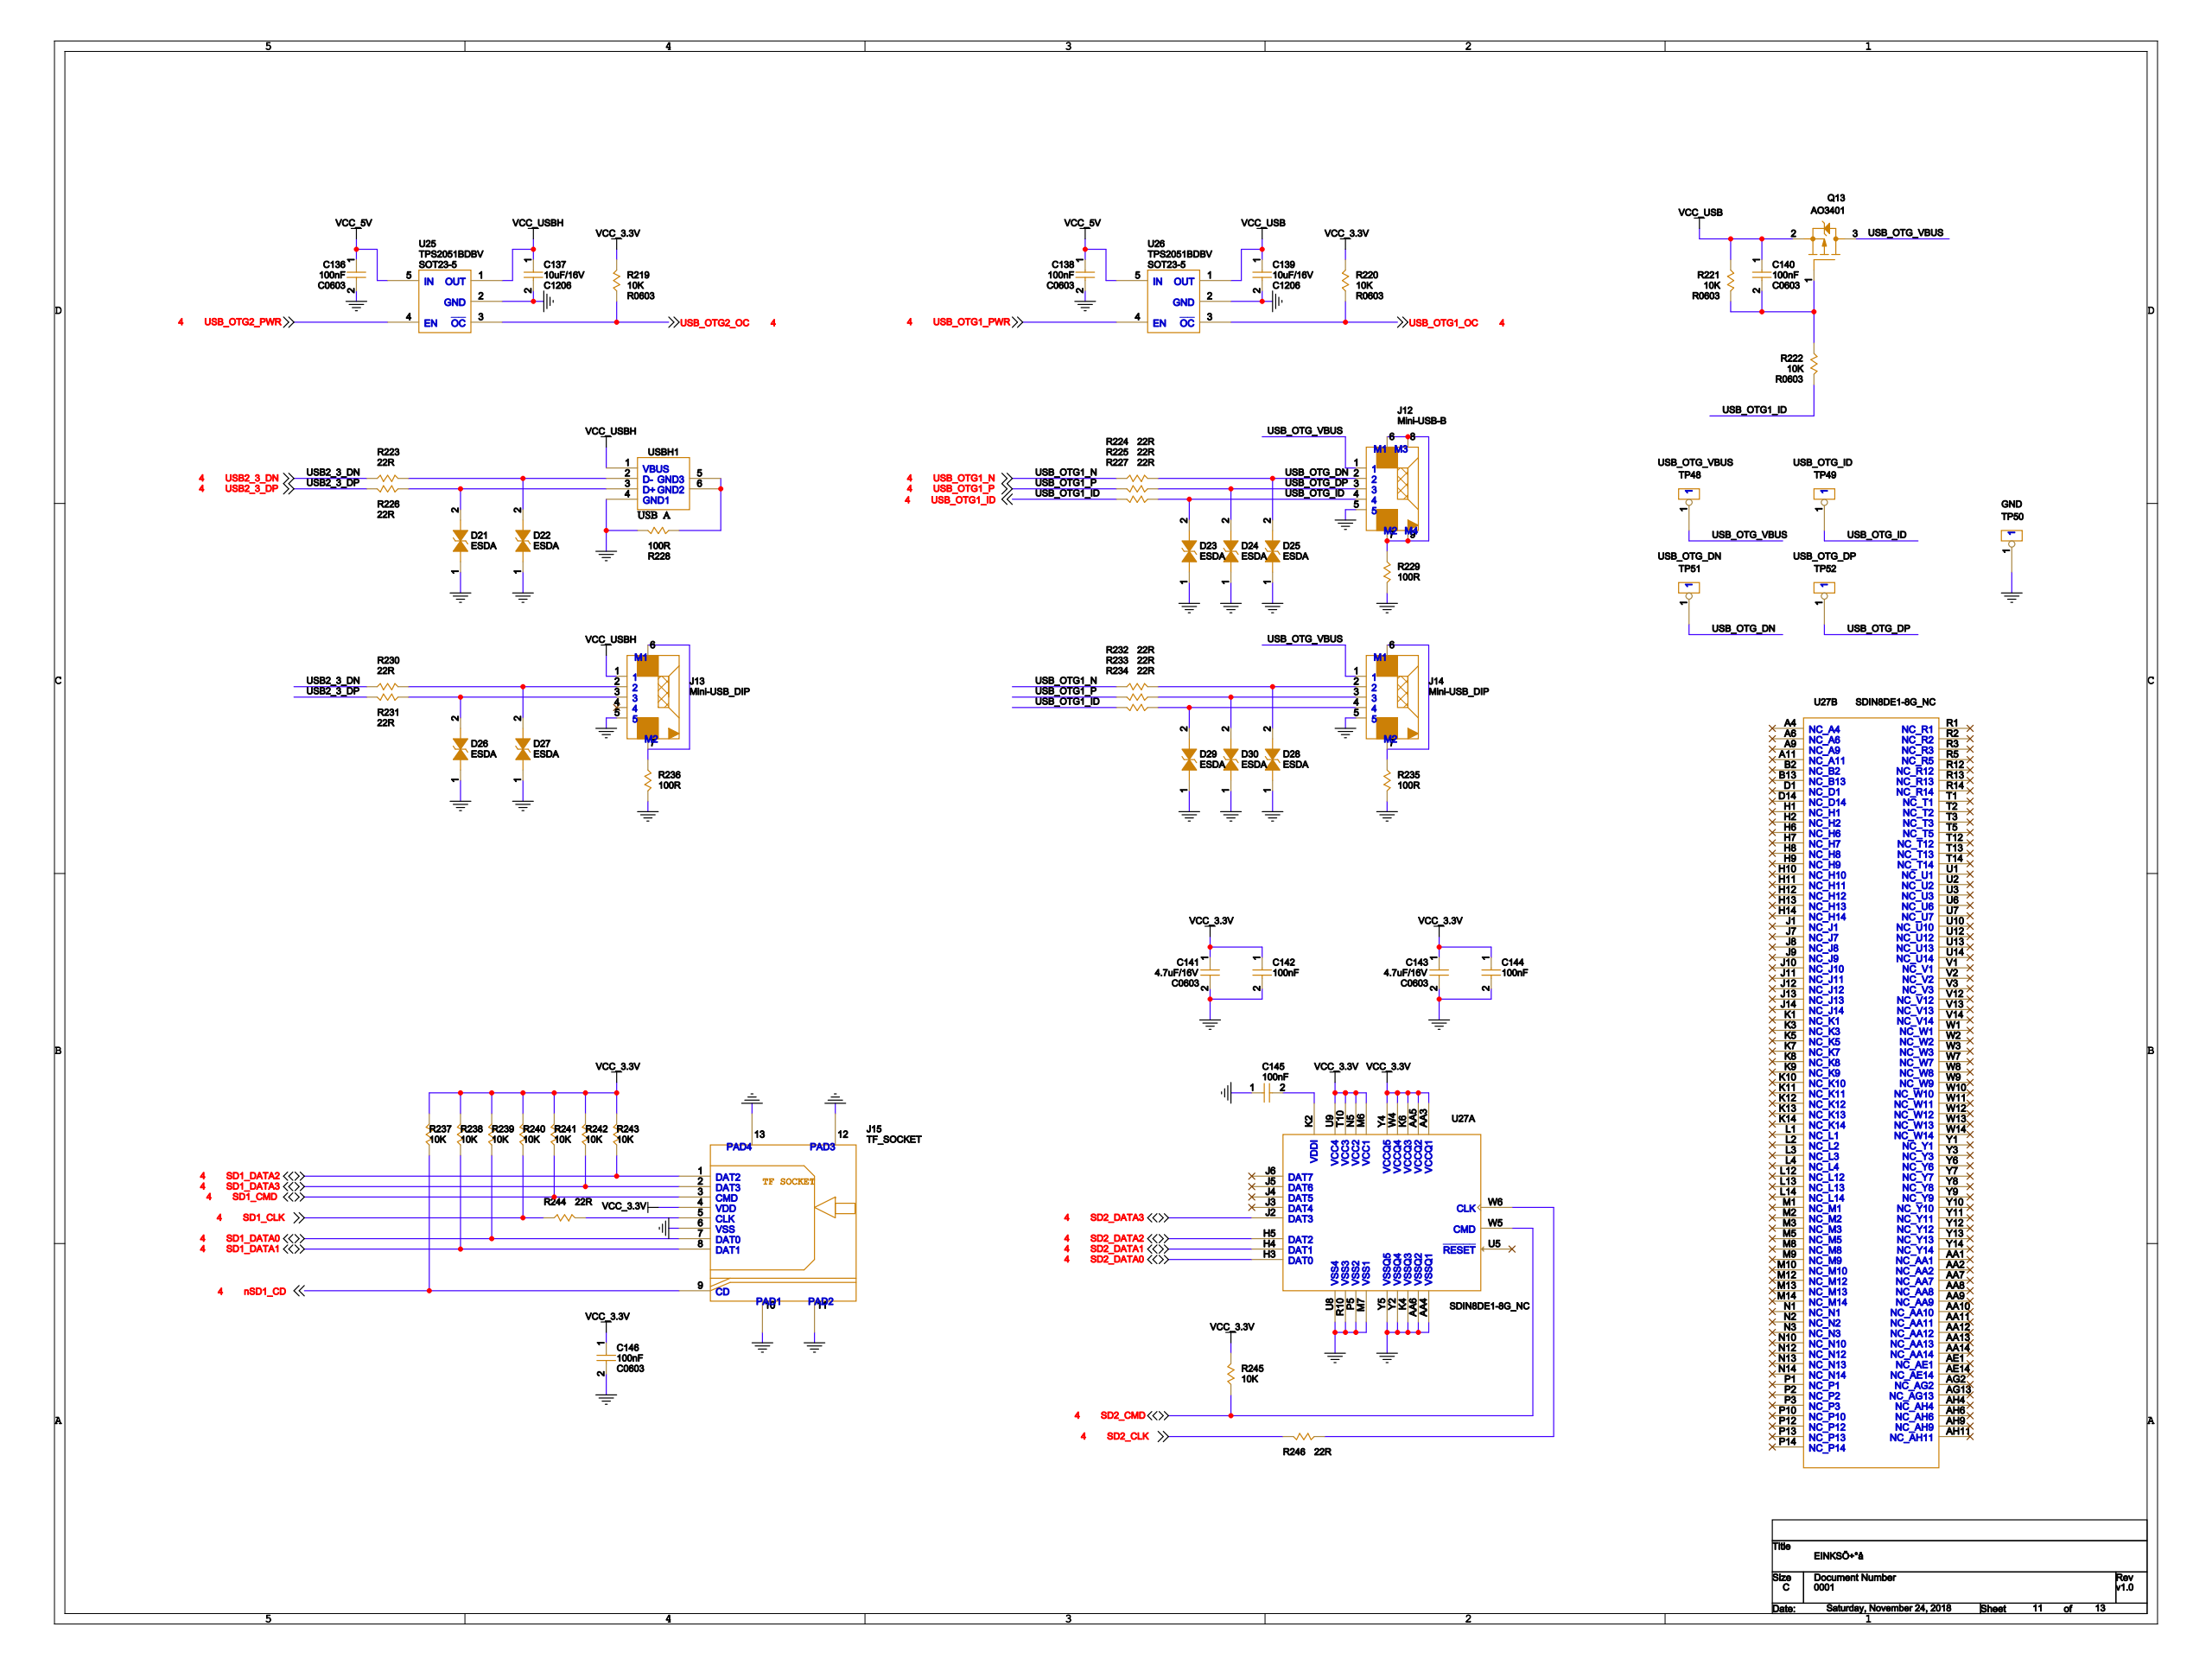Circuit board | Cadence Allegro | 609 parts | 409 nets | one sheet of the schematic
Parts on this sheet (reference | value | footprint):
C136 | 100nF | C0603
C137 | 10uF/16V | C1206
C138 | 100nF | C0603
C139 | 10uF/16V | C1206
C140 | 100nF | C0603
C141 | 4.7uF/16V | C0603
C142 | 100nF | C0603
C143 | 4.7uF/16V | C0603
C144 | 100nF | C0603
C145 | 100nF | C0603
C146 | 100nF | C0603
D21 | ESDA | 0603ESDA
D22 | ESDA | 0603ESDA
D23 | ESDA | 0603ESDA
D24 | ESDA | 0603ESDA
D25 | ESDA | 0603ESDA
D26 | ESDA | 0603ESDA
D27 | ESDA | 0603ESDA
D28 | ESDA | 0603ESDA
D29 | ESDA | 0603ESDA
D30 | ESDA | 0603ESDA
J3 | SAIL_i.MX7D | DDR4_SLT_RVS
J7 | ZIF_FPC_39pin | 39FXL
J12 | Mini-USB-B | MINI_USB_B
J13 | Mini-USB_DIP | MICRO_USB_BS
J14 | Mini-USB_DIP | MICRO_USB_BS
J15 | TF_SOCKET | TF_001
Q13 | AO3401 | SOT23
R219 | 10K | R0603
R220 | 10K | R0603
R221 | 10K | R0603
R222 | 10K | R0603
R223 | 22R | R0603
R224 | 22R | R0603
R225 | 22R | R0603
R226 | 22R | R0603
R227 | 22R | R0603
R228 | 100R | R0603
R229 | 100R | R0603
R230 | 22R | R0603
R231 | 22R | R0603
R232 | 22R | R0603
R233 | 22R | R0603
R234 | 22R | R0603
R235 | 100R | R0603
R236 | 100R | R0603
R237 | 10K | R0603
R238 | 10K | R0603
R239 | 10K | R0603
R240 | 10K | R0603
R241 | 10K | R0603
R242 | 10K | R0603
R243 | 10K | R0603
R244 | 22R | R0603
R245 | 10K | R0603
R246 | 22R | R0603
TP48 | USB_OTG_VBUS | TP_50
TP49 | USB_OTG_ID | TP_50
TP50 | GND | TP_50
TP51 | USB_OTG_DN | TP_50
TP52 | USB_OTG_DP | TP_50
U7 | USB2514B | SQFN36
U8 | SGM8621XN5/TR | SOT23-5
U13 | AR8033 | QFN48P
U25 | TPS2051BDBV | SOT23-5
U26 | TPS2051BDBV | SOT23-5
U27 | SDIN8DE1-8G_NC | BGA169_0P5_12X16
USBH1 | USB  A | USB-A2
Nets of these parts (net: part-pin ...):
VCC_USBH: C137-1 J13-1 U25-1 USBH1-1
N29245546: D27-2 J13-2 R230-1
N29245549: D26-2 J13-3 R231-1
GND: C136-2 C137-2 C138-2 C139-2 C141-2 C142-2 C143-2 C144-2 C145-1 C146-2 D21-1 D22-1 D23-1 D24-1 D25-1 D26-1 D27-1 D28-1 D29-1 D30-1 J12-5 J13-5 J14-5 J15-6 J15-10 J15-11 J15-12 J15-13 R228-2 R229-2 R235-2 R236-2 TP50-1 U8-2 U25-2 U26-2 USBH1-4 J3-1 J3-24 J7-3 J7-8 J7-9 U27-AA4 U27-AA6 U27-K4 U27-M7 U27-P5 U27-R10 U27-U8 U27-Y2 U27-Y5
N29245085: J13-6 J13-7 R236-1
USB_OTG_VBUS: J12-1 J14-1 Q13-3 TP48-1
N29246002: D28-2 J14-2 R232-1
N29246005: D30-2 J14-3 R233-1
N29246008: D29-2 J14-4 R234-1
N29245235: J14-6 J14-7 R235-1
VCC_3.3V: C141-1 C142-1 C143-1 C144-1 C146-1 J15-4 R219-2 R220-2 R237-2 R238-2 R239-2 R240-2 R241-2 R242-2 R243-2 R245-2 U8-5 U7-5 U7-10 U13-4 U27-AA3 U27-AA5 U27-K6 U27-M6 U27-N5 U27-T10 U27-U9 U27-W4 U27-Y4
VCC_5V: C136-1 C138-1 U25-5 U26-5 J3-2 J3-4 J3-6 J3-8 J3-10 J3-12
N28910865: D21-2 R226-1 USBH1-3
N28910861: D22-2 R223-1 USBH1-2
USB_OTG_ID: D23-2 J12-4 R227-1 TP49-1
USB_OTG_DP: D24-2 J12-3 R225-1 TP52-1
USB_OTG_DN: D25-2 J12-2 R224-1 TP51-1
N28912645: J12-6 J12-7 J12-8 J12-9 R229-1
NSD1_CD: J15-9 R237-1
N29231676: J15-5 R244-1
SD1_CMD: J15-3 R241-1
SD1_DATA0: J15-7 R239-1
SD1_DATA1: J15-8 R238-1
SD1_DATA2: J15-1 R243-1
SD1_DATA3: J15-2 R242-1
SD1_CLK: R240-1 R244-2
SD2_CLK: R246-2
SD2_CMD: R245-1 U27-W5
SD2_DATA0: U27-H3
SD2_DATA1: U27-H4
SD2_DATA2: U27-H5
SD2_DATA3: U27-J2
USB_OTG1_ID: R222-1 R227-2 R234-2
USB_OTG1_N: R224-2 R232-2
USB_OTG1_OC: R220-1 U26-3
USB_OTG1_P: R225-2 R233-2
USB_OTG1_PWR: U26-4
USB_OTG2_OC: R219-1 U25-3
USB_OTG2_PWR: U25-4
ADC_BAT_AIN2: U8-1 U8-4
VCC_USB: C139-1 C140-1 Q13-2 R221-2 U26-1
N28926832: R246-1 U27-W6
N28927135: C145-2 U27-K2
USB2_3_DN: R223-2 R230-2 U7-6
USB2_3_DP: R226-2 R231-2 U7-7
N28737112: U8-3
N28914395: C140-2 Q13-1 R221-1 R222-2
N28910817: R228-1 USBH1-5 USBH1-6